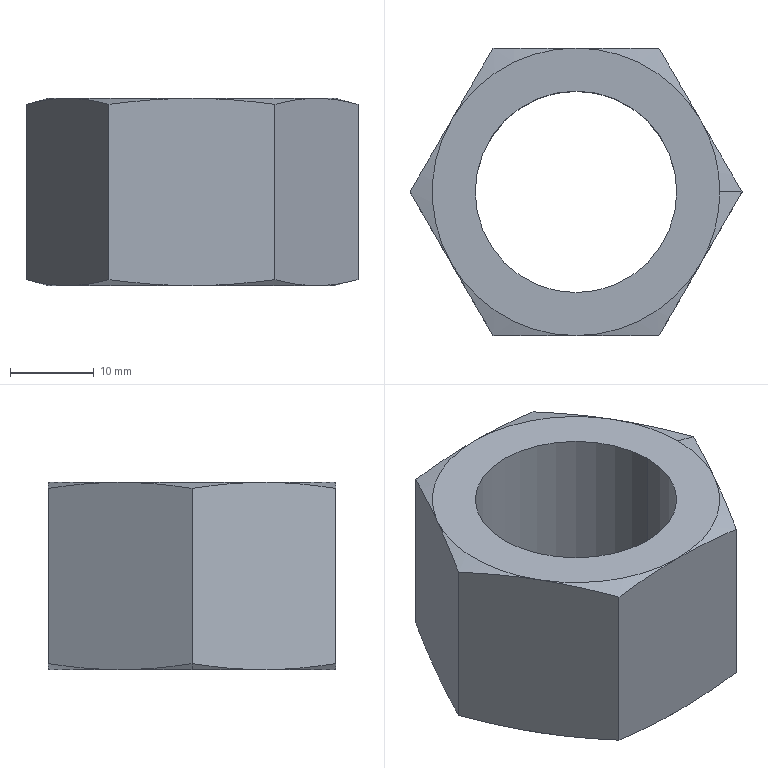Part | SolidWorks | features Cut 2, Chamfer 1, Extrusion 1 | 1 solid | 24 faces | box 39.55 x 34.251 x 22.3 mm | volume 12527 mm3 | cone 14 | plane 8 | cylinder 2 | commonest cylinder face diameters 24 x2
STEP:
#1=CARTESIAN_POINT('',(14.831,8.563,22.3));
#2=VERTEX_POINT('',#1);
#3=CARTESIAN_POINT('',(17.126,0.,22.3));
#4=VERTEX_POINT('',#3);
#5=CARTESIAN_POINT('',(0.,0.,22.3));
#6=DIRECTION('',(0.,0.,-1.));
#7=DIRECTION('',(-1.,0.,0.));
#8=AXIS2_PLACEMENT_3D('',#5,#6,#7);
#9=CIRCLE('',#8,17.126);
#10=EDGE_CURVE('',#2,#4,#9,.T.);
#11=ORIENTED_EDGE('',*,*,#10,.T.);
#12=CARTESIAN_POINT('',(19.775,0.,21.59));
#13=VERTEX_POINT('',#12);
#14=CARTESIAN_POINT('',(17.126,0.,22.3));
#15=DIRECTION('',(0.9659,0.,-0.2588));
#16=VECTOR('',#15,1000.);
#17=LINE('',#14,#16);
#18=EDGE_CURVE('',#4,#13,#17,.T.);
#19=ORIENTED_EDGE('',*,*,#18,.T.);
#20=CARTESIAN_POINT('',(19.775,0.,21.59));
#21=CARTESIAN_POINT('',(18.951,1.427,21.811));
#22=CARTESIAN_POINT('',(18.127,2.854,21.99));
#23=CARTESIAN_POINT('',(16.479,5.709,22.235));
#24=CARTESIAN_POINT('',(15.655,7.136,22.3));
#25=CARTESIAN_POINT('',(14.831,8.563,22.3));
#26=B_SPLINE_CURVE_WITH_KNOTS('',3,(#20,#21,#22,#23,#24,#25),.UNSPECIFIED.,.F.,.F.,(4,2,4),(0.000000231,0.004944,0.009888),.UNSPECIFIED.);
#27=EDGE_CURVE('',#13,#2,#26,.T.);
#28=ORIENTED_EDGE('',*,*,#27,.T.);
#29=EDGE_LOOP('',(#11,#19,#28));
#30=FACE_OUTER_BOUND('',#29,.T.);
#31=CARTESIAN_POINT('',(0.,0.,22.3));
#32=DIRECTION('',(0.,0.,-1.));
#33=DIRECTION('',(1.,0.,0.));
#34=AXIS2_PLACEMENT_3D('',#31,#32,#33);
#35=CONICAL_SURFACE('',#34,17.126,1.309);
#36=ADVANCED_FACE('',(#30),#35,.T.);
#37=CARTESIAN_POINT('',(-17.126,0.,0.));
#38=VERTEX_POINT('',#37);
#39=CARTESIAN_POINT('',(-14.831,8.563,0.));
#40=VERTEX_POINT('',#39);
#41=CARTESIAN_POINT('',(0.,0.,0.));
#42=DIRECTION('',(0.,0.,-1.));
#43=DIRECTION('',(-1.,0.,0.));
#44=AXIS2_PLACEMENT_3D('',#41,#42,#43);
#45=CIRCLE('',#44,17.126);
#46=EDGE_CURVE('',#38,#40,#45,.T.);
#47=ORIENTED_EDGE('',*,*,#46,.F.);
#48=CARTESIAN_POINT('',(-19.775,0.,0.7099));
#49=VERTEX_POINT('',#48);
#50=CARTESIAN_POINT('',(-17.126,0.,0.));
#51=DIRECTION('',(-0.9659,0.,0.2588));
#52=VECTOR('',#51,1000.);
#53=LINE('',#50,#52);
#54=EDGE_CURVE('',#38,#49,#53,.T.);
#55=ORIENTED_EDGE('',*,*,#54,.T.);
#56=CARTESIAN_POINT('',(-19.775,0.,0.7099));
#57=CARTESIAN_POINT('',(-18.951,1.427,0.4891));
#58=CARTESIAN_POINT('',(-18.127,2.854,0.3098));
#59=CARTESIAN_POINT('',(-16.479,5.709,0.06491));
#60=CARTESIAN_POINT('',(-15.655,7.136,0.));
#61=CARTESIAN_POINT('',(-14.831,8.563,0.));
#62=B_SPLINE_CURVE_WITH_KNOTS('',3,(#56,#57,#58,#59,#60,#61),.UNSPECIFIED.,.F.,.F.,(4,2,4),(0.000000231,0.004944,0.009888),.UNSPECIFIED.);
#63=EDGE_CURVE('',#49,#40,#62,.T.);
#64=ORIENTED_EDGE('',*,*,#63,.T.);
#65=EDGE_LOOP('',(#47,#55,#64));
#66=FACE_OUTER_BOUND('',#65,.T.);
#67=CARTESIAN_POINT('',(0.,0.,0.));
#68=DIRECTION('',(0.,0.,1.));
#69=DIRECTION('',(-1.,0.,0.));
#70=AXIS2_PLACEMENT_3D('',#67,#68,#69);
#71=CONICAL_SURFACE('',#70,17.126,1.309);
#72=ADVANCED_FACE('',(#66),#71,.T.);
#73=CARTESIAN_POINT('',(-12.,0.,22.3));
#74=VERTEX_POINT('',#73);
#75=CARTESIAN_POINT('',(12.,0.,22.3));
#76=VERTEX_POINT('',#75);
#77=CARTESIAN_POINT('',(0.,0.,22.3));
#78=DIRECTION('',(0.,0.,1.));
#79=DIRECTION('',(1.,0.,0.));
#80=AXIS2_PLACEMENT_3D('',#77,#78,#79);
#81=CIRCLE('',#80,12.);
#82=EDGE_CURVE('',#74,#76,#81,.T.);
#83=ORIENTED_EDGE('',*,*,#82,.T.);
#84=CARTESIAN_POINT('',(12.,0.,0.));
#85=VERTEX_POINT('',#84);
#86=CARTESIAN_POINT('',(12.,0.,22.3));
#87=DIRECTION('',(0.,0.,-1.));
#88=VECTOR('',#87,1000.);
#89=LINE('',#86,#88);
#90=EDGE_CURVE('',#76,#85,#89,.T.);
#91=ORIENTED_EDGE('',*,*,#90,.T.);
#92=CARTESIAN_POINT('',(-12.,0.,0.));
#93=VERTEX_POINT('',#92);
#94=CARTESIAN_POINT('',(0.,0.,0.));
#95=DIRECTION('',(0.,0.,1.));
#96=DIRECTION('',(1.,0.,0.));
#97=AXIS2_PLACEMENT_3D('',#94,#95,#96);
#98=CIRCLE('',#97,12.);
#99=EDGE_CURVE('',#93,#85,#98,.T.);
#100=ORIENTED_EDGE('',*,*,#99,.F.);
#101=CARTESIAN_POINT('',(-12.,0.,22.3));
#102=DIRECTION('',(0.,0.,-1.));
#103=VECTOR('',#102,1000.);
#104=LINE('',#101,#103);
#105=EDGE_CURVE('',#74,#93,#104,.T.);
#106=ORIENTED_EDGE('',*,*,#105,.F.);
#107=EDGE_LOOP('',(#83,#91,#100,#106));
#108=FACE_OUTER_BOUND('',#107,.T.);
#109=CARTESIAN_POINT('',(0.,0.,22.3));
#110=DIRECTION('',(0.,0.,-1.));
#111=DIRECTION('',(-1.,0.,0.));
#112=AXIS2_PLACEMENT_3D('',#109,#110,#111);
#113=CYLINDRICAL_SURFACE('',#112,12.);
#114=ADVANCED_FACE('',(#108),#113,.F.);
#115=ORIENTED_EDGE('',*,*,#27,.F.);
#116=CARTESIAN_POINT('',(19.775,0.,0.7099));
#117=VERTEX_POINT('',#116);
#118=CARTESIAN_POINT('',(19.775,0.,22.3));
#119=DIRECTION('',(0.,0.,-1.));
#120=VECTOR('',#119,1000.);
#121=LINE('',#118,#120);
#122=EDGE_CURVE('',#13,#117,#121,.T.);
#123=ORIENTED_EDGE('',*,*,#122,.T.);
#124=CARTESIAN_POINT('',(14.831,8.563,0.));
#125=VERTEX_POINT('',#124);
#126=CARTESIAN_POINT('',(14.831,8.563,0.));
#127=CARTESIAN_POINT('',(15.655,7.136,0.));
#128=CARTESIAN_POINT('',(16.479,5.709,0.06491));
#129=CARTESIAN_POINT('',(18.127,2.854,0.3098));
#130=CARTESIAN_POINT('',(18.951,1.427,0.4891));
#131=CARTESIAN_POINT('',(19.775,0.,0.7099));
#132=B_SPLINE_CURVE_WITH_KNOTS('',3,(#126,#127,#128,#129,#130,#131),.UNSPECIFIED.,.F.,.F.,(4,2,4),(0.009888,0.01483,0.01978),.UNSPECIFIED.);
#133=EDGE_CURVE('',#125,#117,#132,.T.);
#134=ORIENTED_EDGE('',*,*,#133,.F.);
#135=CARTESIAN_POINT('',(9.888,17.126,0.7099));
#136=VERTEX_POINT('',#135);
#137=CARTESIAN_POINT('',(9.888,17.126,0.7099));
#138=CARTESIAN_POINT('',(10.711,15.699,0.4891));
#139=CARTESIAN_POINT('',(11.535,14.271,0.3098));
#140=CARTESIAN_POINT('',(13.183,11.417,0.06491));
#141=CARTESIAN_POINT('',(14.007,9.99,0.));
#142=CARTESIAN_POINT('',(14.831,8.563,0.));
#143=B_SPLINE_CURVE_WITH_KNOTS('',3,(#137,#138,#139,#140,#141,#142),.UNSPECIFIED.,.F.,.F.,(4,2,4),(0.000000231,0.004944,0.009888),.UNSPECIFIED.);
#144=EDGE_CURVE('',#136,#125,#143,.T.);
#145=ORIENTED_EDGE('',*,*,#144,.F.);
#146=CARTESIAN_POINT('',(9.888,17.126,21.59));
#147=VERTEX_POINT('',#146);
#148=CARTESIAN_POINT('',(9.888,17.126,22.3));
#149=DIRECTION('',(0.,0.,-1.));
#150=VECTOR('',#149,1000.);
#151=LINE('',#148,#150);
#152=EDGE_CURVE('',#147,#136,#151,.T.);
#153=ORIENTED_EDGE('',*,*,#152,.F.);
#154=CARTESIAN_POINT('',(14.831,8.563,22.3));
#155=CARTESIAN_POINT('',(14.007,9.99,22.3));
#156=CARTESIAN_POINT('',(13.183,11.417,22.235));
#157=CARTESIAN_POINT('',(11.535,14.271,21.99));
#158=CARTESIAN_POINT('',(10.711,15.699,21.811));
#159=CARTESIAN_POINT('',(9.888,17.126,21.59));
#160=B_SPLINE_CURVE_WITH_KNOTS('',3,(#154,#155,#156,#157,#158,#159),.UNSPECIFIED.,.F.,.F.,(4,2,4),(0.009888,0.01483,0.01978),.UNSPECIFIED.);
#161=EDGE_CURVE('',#2,#147,#160,.T.);
#162=ORIENTED_EDGE('',*,*,#161,.F.);
#163=EDGE_LOOP('',(#115,#123,#134,#145,#153,#162));
#164=FACE_OUTER_BOUND('',#163,.T.);
#165=CARTESIAN_POINT('',(19.775,0.,22.3));
#166=DIRECTION('',(-0.866,-0.5,0.));
#167=DIRECTION('',(0.5,-0.866,0.));
#168=AXIS2_PLACEMENT_3D('',#165,#166,#167);
#169=PLANE('',#168);
#170=ADVANCED_FACE('',(#164),#169,.F.);
#171=CARTESIAN_POINT('',(0.,17.126,22.3));
#172=VERTEX_POINT('',#171);
#173=CARTESIAN_POINT('',(9.888,17.126,21.59));
#174=CARTESIAN_POINT('',(8.242,17.126,21.811));
#175=CARTESIAN_POINT('',(6.596,17.126,21.99));
#176=CARTESIAN_POINT('',(3.3,17.126,22.235));
#177=CARTESIAN_POINT('',(1.651,17.126,22.3));
#178=CARTESIAN_POINT('',(0.,17.126,22.3));
#179=B_SPLINE_CURVE_WITH_KNOTS('',3,(#173,#174,#175,#176,#177,#178),.UNSPECIFIED.,.F.,.F.,(4,2,4),(0.05691,0.06188,0.06685),.UNSPECIFIED.);
#180=EDGE_CURVE('',#147,#172,#179,.T.);
#181=ORIENTED_EDGE('',*,*,#180,.F.);
#182=ORIENTED_EDGE('',*,*,#152,.T.);
#183=CARTESIAN_POINT('',(0.,17.126,0.));
#184=VERTEX_POINT('',#183);
#185=CARTESIAN_POINT('',(0.,17.126,0.));
#186=CARTESIAN_POINT('',(1.651,17.126,0.));
#187=CARTESIAN_POINT('',(3.3,17.126,0.06515));
#188=CARTESIAN_POINT('',(6.596,17.126,0.3103));
#189=CARTESIAN_POINT('',(8.242,17.126,0.4895));
#190=CARTESIAN_POINT('',(9.888,17.126,0.7099));
#191=B_SPLINE_CURVE_WITH_KNOTS('',3,(#185,#186,#187,#188,#189,#190),.UNSPECIFIED.,.F.,.F.,(4,2,4),(0.02684,0.03182,0.03681),.UNSPECIFIED.);
#192=EDGE_CURVE('',#184,#136,#191,.T.);
#193=ORIENTED_EDGE('',*,*,#192,.F.);
#194=CARTESIAN_POINT('',(-9.887,17.126,0.7099));
#195=VERTEX_POINT('',#194);
#196=CARTESIAN_POINT('',(-9.887,17.126,0.7099));
#197=CARTESIAN_POINT('',(-8.244,17.126,0.4897));
#198=CARTESIAN_POINT('',(-6.591,17.126,0.3098));
#199=CARTESIAN_POINT('',(-3.293,17.126,0.06475));
#200=CARTESIAN_POINT('',(-1.646,17.126,0.));
#201=CARTESIAN_POINT('',(0.,17.126,0.));
#202=B_SPLINE_CURVE_WITH_KNOTS('',3,(#196,#197,#198,#199,#200,#201),.UNSPECIFIED.,.F.,.F.,(4,2,4),(0.0169,0.02187,0.02684),.UNSPECIFIED.);
#203=EDGE_CURVE('',#195,#184,#202,.T.);
#204=ORIENTED_EDGE('',*,*,#203,.F.);
#205=CARTESIAN_POINT('',(-9.887,17.126,21.59));
#206=VERTEX_POINT('',#205);
#207=CARTESIAN_POINT('',(-9.887,17.126,22.3));
#208=DIRECTION('',(0.,0.,-1.));
#209=VECTOR('',#208,1000.);
#210=LINE('',#207,#209);
#211=EDGE_CURVE('',#206,#195,#210,.T.);
#212=ORIENTED_EDGE('',*,*,#211,.F.);
#213=CARTESIAN_POINT('',(0.,17.126,22.3));
#214=CARTESIAN_POINT('',(-1.646,17.126,22.3));
#215=CARTESIAN_POINT('',(-3.293,17.126,22.235));
#216=CARTESIAN_POINT('',(-6.591,17.126,21.99));
#217=CARTESIAN_POINT('',(-8.244,17.126,21.81));
#218=CARTESIAN_POINT('',(-9.887,17.126,21.59));
#219=B_SPLINE_CURVE_WITH_KNOTS('',3,(#213,#214,#215,#216,#217,#218),.UNSPECIFIED.,.F.,.F.,(4,2,4),(0.06685,0.07181,0.07677),.UNSPECIFIED.);
#220=EDGE_CURVE('',#172,#206,#219,.T.);
#221=ORIENTED_EDGE('',*,*,#220,.F.);
#222=EDGE_LOOP('',(#181,#182,#193,#204,#212,#221));
#223=FACE_OUTER_BOUND('',#222,.T.);
#224=CARTESIAN_POINT('',(9.888,17.126,22.3));
#225=DIRECTION('',(0.,-1.,0.));
#226=DIRECTION('',(1.,0.,0.));
#227=AXIS2_PLACEMENT_3D('',#224,#225,#226);
#228=PLANE('',#227);
#229=ADVANCED_FACE('',(#223),#228,.F.);
#230=CARTESIAN_POINT('',(-14.831,8.563,22.3));
#231=VERTEX_POINT('',#230);
#232=CARTESIAN_POINT('',(-9.887,17.126,21.59));
#233=CARTESIAN_POINT('',(-10.711,15.699,21.811));
#234=CARTESIAN_POINT('',(-11.535,14.271,21.99));
#235=CARTESIAN_POINT('',(-13.183,11.417,22.235));
#236=CARTESIAN_POINT('',(-14.007,9.99,22.3));
#237=CARTESIAN_POINT('',(-14.831,8.563,22.3));
#238=B_SPLINE_CURVE_WITH_KNOTS('',3,(#232,#233,#234,#235,#236,#237),.UNSPECIFIED.,.F.,.F.,(4,2,4),(0.000000231,0.004944,0.009888),.UNSPECIFIED.);
#239=EDGE_CURVE('',#206,#231,#238,.T.);
#240=ORIENTED_EDGE('',*,*,#239,.F.);
#241=ORIENTED_EDGE('',*,*,#211,.T.);
#242=CARTESIAN_POINT('',(-14.831,8.563,0.));
#243=CARTESIAN_POINT('',(-14.007,9.99,0.));
#244=CARTESIAN_POINT('',(-13.183,11.417,0.06491));
#245=CARTESIAN_POINT('',(-11.535,14.271,0.3098));
#246=CARTESIAN_POINT('',(-10.711,15.699,0.4891));
#247=CARTESIAN_POINT('',(-9.887,17.126,0.7099));
#248=B_SPLINE_CURVE_WITH_KNOTS('',3,(#242,#243,#244,#245,#246,#247),.UNSPECIFIED.,.F.,.F.,(4,2,4),(0.009888,0.01483,0.01978),.UNSPECIFIED.);
#249=EDGE_CURVE('',#40,#195,#248,.T.);
#250=ORIENTED_EDGE('',*,*,#249,.F.);
#251=ORIENTED_EDGE('',*,*,#63,.F.);
#252=CARTESIAN_POINT('',(-19.775,0.,21.59));
#253=VERTEX_POINT('',#252);
#254=CARTESIAN_POINT('',(-19.775,0.,22.3));
#255=DIRECTION('',(0.,0.,-1.));
#256=VECTOR('',#255,1000.);
#257=LINE('',#254,#256);
#258=EDGE_CURVE('',#253,#49,#257,.T.);
#259=ORIENTED_EDGE('',*,*,#258,.F.);
#260=CARTESIAN_POINT('',(-14.831,8.563,22.3));
#261=CARTESIAN_POINT('',(-15.655,7.136,22.3));
#262=CARTESIAN_POINT('',(-16.479,5.709,22.235));
#263=CARTESIAN_POINT('',(-18.127,2.854,21.99));
#264=CARTESIAN_POINT('',(-18.951,1.427,21.811));
#265=CARTESIAN_POINT('',(-19.775,0.,21.59));
#266=B_SPLINE_CURVE_WITH_KNOTS('',3,(#260,#261,#262,#263,#264,#265),.UNSPECIFIED.,.F.,.F.,(4,2,4),(0.009888,0.01483,0.01978),.UNSPECIFIED.);
#267=EDGE_CURVE('',#231,#253,#266,.T.);
#268=ORIENTED_EDGE('',*,*,#267,.F.);
#269=EDGE_LOOP('',(#240,#241,#250,#251,#259,#268));
#270=FACE_OUTER_BOUND('',#269,.T.);
#271=CARTESIAN_POINT('',(-9.887,17.126,22.3));
#272=DIRECTION('',(0.866,-0.5,0.));
#273=DIRECTION('',(0.5,0.866,0.));
#274=AXIS2_PLACEMENT_3D('',#271,#272,#273);
#275=PLANE('',#274);
#276=ADVANCED_FACE('',(#270),#275,.F.);
#277=CARTESIAN_POINT('',(-14.831,-8.563,22.3));
#278=VERTEX_POINT('',#277);
#279=CARTESIAN_POINT('',(-19.775,0.,21.59));
#280=CARTESIAN_POINT('',(-18.951,-1.427,21.811));
#281=CARTESIAN_POINT('',(-18.127,-2.854,21.99));
#282=CARTESIAN_POINT('',(-16.479,-5.709,22.235));
#283=CARTESIAN_POINT('',(-15.655,-7.136,22.3));
#284=CARTESIAN_POINT('',(-14.831,-8.563,22.3));
#285=B_SPLINE_CURVE_WITH_KNOTS('',3,(#279,#280,#281,#282,#283,#284),.UNSPECIFIED.,.F.,.F.,(4,2,4),(0.000000231,0.004944,0.009888),.UNSPECIFIED.);
#286=EDGE_CURVE('',#253,#278,#285,.T.);
#287=ORIENTED_EDGE('',*,*,#286,.F.);
#288=ORIENTED_EDGE('',*,*,#258,.T.);
#289=CARTESIAN_POINT('',(-14.831,-8.563,0.));
#290=VERTEX_POINT('',#289);
#291=CARTESIAN_POINT('',(-14.831,-8.563,0.));
#292=CARTESIAN_POINT('',(-15.655,-7.136,0.));
#293=CARTESIAN_POINT('',(-16.479,-5.709,0.06491));
#294=CARTESIAN_POINT('',(-18.127,-2.854,0.3098));
#295=CARTESIAN_POINT('',(-18.951,-1.427,0.4891));
#296=CARTESIAN_POINT('',(-19.775,0.,0.7099));
#297=B_SPLINE_CURVE_WITH_KNOTS('',3,(#291,#292,#293,#294,#295,#296),.UNSPECIFIED.,.F.,.F.,(4,2,4),(0.009888,0.01483,0.01978),.UNSPECIFIED.);
#298=EDGE_CURVE('',#290,#49,#297,.T.);
#299=ORIENTED_EDGE('',*,*,#298,.F.);
#300=CARTESIAN_POINT('',(-9.887,-17.126,0.7099));
#301=VERTEX_POINT('',#300);
#302=CARTESIAN_POINT('',(-9.887,-17.126,0.7099));
#303=CARTESIAN_POINT('',(-10.711,-15.699,0.4891));
#304=CARTESIAN_POINT('',(-11.535,-14.271,0.3098));
#305=CARTESIAN_POINT('',(-13.183,-11.417,0.06491));
#306=CARTESIAN_POINT('',(-14.007,-9.99,0.));
#307=CARTESIAN_POINT('',(-14.831,-8.563,0.));
#308=B_SPLINE_CURVE_WITH_KNOTS('',3,(#302,#303,#304,#305,#306,#307),.UNSPECIFIED.,.F.,.F.,(4,2,4),(0.000000231,0.004944,0.009888),.UNSPECIFIED.);
#309=EDGE_CURVE('',#301,#290,#308,.T.);
#310=ORIENTED_EDGE('',*,*,#309,.F.);
#311=CARTESIAN_POINT('',(-9.887,-17.126,21.59));
#312=VERTEX_POINT('',#311);
#313=CARTESIAN_POINT('',(-9.887,-17.126,22.3));
#314=DIRECTION('',(0.,0.,-1.));
#315=VECTOR('',#314,1000.);
#316=LINE('',#313,#315);
#317=EDGE_CURVE('',#312,#301,#316,.T.);
#318=ORIENTED_EDGE('',*,*,#317,.F.);
#319=CARTESIAN_POINT('',(-14.831,-8.563,22.3));
#320=CARTESIAN_POINT('',(-14.007,-9.99,22.3));
#321=CARTESIAN_POINT('',(-13.183,-11.417,22.235));
#322=CARTESIAN_POINT('',(-11.535,-14.271,21.99));
#323=CARTESIAN_POINT('',(-10.711,-15.699,21.811));
#324=CARTESIAN_POINT('',(-9.887,-17.126,21.59));
#325=B_SPLINE_CURVE_WITH_KNOTS('',3,(#319,#320,#321,#322,#323,#324),.UNSPECIFIED.,.F.,.F.,(4,2,4),(0.009888,0.01483,0.01978),.UNSPECIFIED.);
#326=EDGE_CURVE('',#278,#312,#325,.T.);
#327=ORIENTED_EDGE('',*,*,#326,.F.);
#328=EDGE_LOOP('',(#287,#288,#299,#310,#318,#327));
#329=FACE_OUTER_BOUND('',#328,.T.);
#330=CARTESIAN_POINT('',(-19.775,0.,22.3));
#331=DIRECTION('',(0.866,0.5,0.));
#332=DIRECTION('',(-0.5,0.866,0.));
#333=AXIS2_PLACEMENT_3D('',#330,#331,#332);
#334=PLANE('',#333);
#335=ADVANCED_FACE('',(#329),#334,.F.);
#336=CARTESIAN_POINT('',(0.,-17.126,22.3));
#337=VERTEX_POINT('',#336);
#338=CARTESIAN_POINT('',(-9.887,-17.126,21.59));
#339=CARTESIAN_POINT('',(-8.244,-17.126,21.81));
#340=CARTESIAN_POINT('',(-6.591,-17.126,21.99));
#341=CARTESIAN_POINT('',(-3.293,-17.126,22.235));
#342=CARTESIAN_POINT('',(-1.646,-17.126,22.3));
#343=CARTESIAN_POINT('',(0.,-17.126,22.3));
#344=B_SPLINE_CURVE_WITH_KNOTS('',3,(#338,#339,#340,#341,#342,#343),.UNSPECIFIED.,.F.,.F.,(4,2,4),(0.0169,0.02187,0.02684),.UNSPECIFIED.);
#345=EDGE_CURVE('',#312,#337,#344,.T.);
#346=ORIENTED_EDGE('',*,*,#345,.F.);
#347=ORIENTED_EDGE('',*,*,#317,.T.);
#348=CARTESIAN_POINT('',(0.,-17.126,0.));
#349=VERTEX_POINT('',#348);
#350=CARTESIAN_POINT('',(0.,-17.126,0.));
#351=CARTESIAN_POINT('',(-1.646,-17.126,0.));
#352=CARTESIAN_POINT('',(-3.293,-17.126,0.06475));
#353=CARTESIAN_POINT('',(-6.591,-17.126,0.3098));
#354=CARTESIAN_POINT('',(-8.244,-17.126,0.4897));
#355=CARTESIAN_POINT('',(-9.887,-17.126,0.7099));
#356=B_SPLINE_CURVE_WITH_KNOTS('',3,(#350,#351,#352,#353,#354,#355),.UNSPECIFIED.,.F.,.F.,(4,2,4),(0.06685,0.07181,0.07677),.UNSPECIFIED.);
#357=EDGE_CURVE('',#349,#301,#356,.T.);
#358=ORIENTED_EDGE('',*,*,#357,.F.);
#359=CARTESIAN_POINT('',(9.887,-17.126,0.7099));
#360=VERTEX_POINT('',#359);
#361=CARTESIAN_POINT('',(9.887,-17.126,0.7099));
#362=CARTESIAN_POINT('',(8.242,-17.126,0.4895));
#363=CARTESIAN_POINT('',(6.596,-17.126,0.3103));
#364=CARTESIAN_POINT('',(3.3,-17.126,0.06515));
#365=CARTESIAN_POINT('',(1.651,-17.126,0.));
#366=CARTESIAN_POINT('',(0.,-17.126,0.));
#367=B_SPLINE_CURVE_WITH_KNOTS('',3,(#361,#362,#363,#364,#365,#366),.UNSPECIFIED.,.F.,.F.,(4,2,4),(0.05691,0.06188,0.06685),.UNSPECIFIED.);
#368=EDGE_CURVE('',#360,#349,#367,.T.);
#369=ORIENTED_EDGE('',*,*,#368,.F.);
#370=CARTESIAN_POINT('',(9.887,-17.126,21.59));
#371=VERTEX_POINT('',#370);
#372=CARTESIAN_POINT('',(9.887,-17.126,22.3));
#373=DIRECTION('',(0.,0.,-1.));
#374=VECTOR('',#373,1000.);
#375=LINE('',#372,#374);
#376=EDGE_CURVE('',#371,#360,#375,.T.);
#377=ORIENTED_EDGE('',*,*,#376,.F.);
#378=CARTESIAN_POINT('',(0.,-17.126,22.3));
#379=CARTESIAN_POINT('',(1.651,-17.126,22.3));
#380=CARTESIAN_POINT('',(3.3,-17.126,22.235));
#381=CARTESIAN_POINT('',(6.596,-17.126,21.99));
#382=CARTESIAN_POINT('',(8.242,-17.126,21.811));
#383=CARTESIAN_POINT('',(9.887,-17.126,21.59));
#384=B_SPLINE_CURVE_WITH_KNOTS('',3,(#378,#379,#380,#381,#382,#383),.UNSPECIFIED.,.F.,.F.,(4,2,4),(0.02684,0.03182,0.03681),.UNSPECIFIED.);
#385=EDGE_CURVE('',#337,#371,#384,.T.);
#386=ORIENTED_EDGE('',*,*,#385,.F.);
#387=EDGE_LOOP('',(#346,#347,#358,#369,#377,#386));
#388=FACE_OUTER_BOUND('',#387,.T.);
#389=CARTESIAN_POINT('',(-9.887,-17.126,22.3));
#390=DIRECTION('',(0.,1.,0.));
#391=DIRECTION('',(-1.,0.,0.));
#392=AXIS2_PLACEMENT_3D('',#389,#390,#391);
#393=PLANE('',#392);
#394=ADVANCED_FACE('',(#388),#393,.F.);
#395=CARTESIAN_POINT('',(14.831,-8.563,22.3));
#396=VERTEX_POINT('',#395);
#397=CARTESIAN_POINT('',(9.887,-17.126,21.59));
#398=CARTESIAN_POINT('',(10.711,-15.699,21.811));
#399=CARTESIAN_POINT('',(11.535,-14.271,21.99));
#400=CARTESIAN_POINT('',(13.183,-11.417,22.235));
#401=CARTESIAN_POINT('',(14.007,-9.99,22.3));
#402=CARTESIAN_POINT('',(14.831,-8.563,22.3));
#403=B_SPLINE_CURVE_WITH_KNOTS('',3,(#397,#398,#399,#400,#401,#402),.UNSPECIFIED.,.F.,.F.,(4,2,4),(0.000000231,0.004944,0.009888),.UNSPECIFIED.);
#404=EDGE_CURVE('',#371,#396,#403,.T.);
#405=ORIENTED_EDGE('',*,*,#404,.F.);
#406=ORIENTED_EDGE('',*,*,#376,.T.);
#407=CARTESIAN_POINT('',(14.831,-8.563,0.));
#408=VERTEX_POINT('',#407);
#409=CARTESIAN_POINT('',(14.831,-8.563,0.));
#410=CARTESIAN_POINT('',(14.007,-9.99,0.));
#411=CARTESIAN_POINT('',(13.183,-11.417,0.06491));
#412=CARTESIAN_POINT('',(11.535,-14.271,0.3098));
#413=CARTESIAN_POINT('',(10.711,-15.699,0.4891));
#414=CARTESIAN_POINT('',(9.887,-17.126,0.7099));
#415=B_SPLINE_CURVE_WITH_KNOTS('',3,(#409,#410,#411,#412,#413,#414),.UNSPECIFIED.,.F.,.F.,(4,2,4),(0.009888,0.01483,0.01978),.UNSPECIFIED.);
#416=EDGE_CURVE('',#408,#360,#415,.T.);
#417=ORIENTED_EDGE('',*,*,#416,.F.);
#418=CARTESIAN_POINT('',(19.775,0.,0.7099));
#419=CARTESIAN_POINT('',(18.951,-1.427,0.4891));
#420=CARTESIAN_POINT('',(18.127,-2.854,0.3098));
#421=CARTESIAN_POINT('',(16.479,-5.709,0.06491));
#422=CARTESIAN_POINT('',(15.655,-7.136,0.));
#423=CARTESIAN_POINT('',(14.831,-8.563,0.));
#424=B_SPLINE_CURVE_WITH_KNOTS('',3,(#418,#419,#420,#421,#422,#423),.UNSPECIFIED.,.F.,.F.,(4,2,4),(0.000000231,0.004944,0.009888),.UNSPECIFIED.);
#425=EDGE_CURVE('',#117,#408,#424,.T.);
#426=ORIENTED_EDGE('',*,*,#425,.F.);
#427=ORIENTED_EDGE('',*,*,#122,.F.);
#428=CARTESIAN_POINT('',(14.831,-8.563,22.3));
#429=CARTESIAN_POINT('',(15.655,-7.136,22.3));
#430=CARTESIAN_POINT('',(16.479,-5.709,22.235));
#431=CARTESIAN_POINT('',(18.127,-2.854,21.99));
#432=CARTESIAN_POINT('',(18.951,-1.427,21.811));
#433=CARTESIAN_POINT('',(19.775,0.,21.59));
#434=B_SPLINE_CURVE_WITH_KNOTS('',3,(#428,#429,#430,#431,#432,#433),.UNSPECIFIED.,.F.,.F.,(4,2,4),(0.009888,0.01483,0.01978),.UNSPECIFIED.);
#435=EDGE_CURVE('',#396,#13,#434,.T.);
#436=ORIENTED_EDGE('',*,*,#435,.F.);
#437=EDGE_LOOP('',(#405,#406,#417,#426,#427,#436));
#438=FACE_OUTER_BOUND('',#437,.T.);
#439=CARTESIAN_POINT('',(9.887,-17.126,22.3));
#440=DIRECTION('',(-0.866,0.5,0.));
#441=DIRECTION('',(-0.5,-0.866,0.));
#442=AXIS2_PLACEMENT_3D('',#439,#440,#441);
#443=PLANE('',#442);
#444=ADVANCED_FACE('',(#438),#443,.F.);
#445=ORIENTED_EDGE('',*,*,#82,.F.);
#446=CARTESIAN_POINT('',(0.,0.,22.3));
#447=DIRECTION('',(0.,0.,1.));
#448=DIRECTION('',(1.,0.,0.));
#449=AXIS2_PLACEMENT_3D('',#446,#447,#448);
#450=CIRCLE('',#449,12.);
#451=EDGE_CURVE('',#76,#74,#450,.T.);
#452=ORIENTED_EDGE('',*,*,#451,.F.);
#453=EDGE_LOOP('',(#445,#452));
#454=FACE_BOUND('',#453,.T.);
#455=CARTESIAN_POINT('',(0.,0.,22.3));
#456=DIRECTION('',(0.,0.,-1.));
#457=DIRECTION('',(-1.,0.,0.));
#458=AXIS2_PLACEMENT_3D('',#455,#456,#457);
#459=CIRCLE('',#458,17.126);
#460=EDGE_CURVE('',#231,#172,#459,.T.);
#461=ORIENTED_EDGE('',*,*,#460,.F.);
#462=CARTESIAN_POINT('',(0.,0.,22.3));
#463=DIRECTION('',(0.,0.,-1.));
#464=DIRECTION('',(-1.,0.,0.));
#465=AXIS2_PLACEMENT_3D('',#462,#463,#464);
#466=CIRCLE('',#465,17.126);
#467=EDGE_CURVE('',#278,#231,#466,.T.);
#468=ORIENTED_EDGE('',*,*,#467,.F.);
#469=CARTESIAN_POINT('',(0.,0.,22.3));
#470=DIRECTION('',(0.,0.,-1.));
#471=DIRECTION('',(-1.,0.,0.));
#472=AXIS2_PLACEMENT_3D('',#469,#470,#471);
#473=CIRCLE('',#472,17.126);
#474=EDGE_CURVE('',#337,#278,#473,.T.);
#475=ORIENTED_EDGE('',*,*,#474,.F.);
#476=CARTESIAN_POINT('',(0.,0.,22.3));
#477=DIRECTION('',(0.,0.,-1.));
#478=DIRECTION('',(-1.,0.,0.));
#479=AXIS2_PLACEMENT_3D('',#476,#477,#478);
#480=CIRCLE('',#479,17.126);
#481=EDGE_CURVE('',#396,#337,#480,.T.);
#482=ORIENTED_EDGE('',*,*,#481,.F.);
#483=CARTESIAN_POINT('',(0.,0.,22.3));
#484=DIRECTION('',(0.,0.,-1.));
#485=DIRECTION('',(-1.,0.,0.));
#486=AXIS2_PLACEMENT_3D('',#483,#484,#485);
#487=CIRCLE('',#486,17.126);
#488=EDGE_CURVE('',#4,#396,#487,.T.);
#489=ORIENTED_EDGE('',*,*,#488,.F.);
#490=ORIENTED_EDGE('',*,*,#10,.F.);
#491=CARTESIAN_POINT('',(0.,0.,22.3));
#492=DIRECTION('',(0.,0.,1.));
#493=DIRECTION('',(1.,0.,0.));
#494=AXIS2_PLACEMENT_3D('',#491,#492,#493);
#495=CIRCLE('',#494,17.126);
#496=EDGE_CURVE('',#2,#172,#495,.T.);
#497=ORIENTED_EDGE('',*,*,#496,.T.);
#498=EDGE_LOOP('',(#461,#468,#475,#482,#489,#490,#497));
#499=FACE_OUTER_BOUND('',#498,.T.);
#500=CARTESIAN_POINT('',(19.775,0.,22.3));
#501=DIRECTION('',(0.,0.,-1.));
#502=DIRECTION('',(-1.,0.,0.));
#503=AXIS2_PLACEMENT_3D('',#500,#501,#502);
#504=PLANE('',#503);
#505=ADVANCED_FACE('',(#454,#499),#504,.F.);
#506=ORIENTED_EDGE('',*,*,#99,.T.);
#507=CARTESIAN_POINT('',(0.,0.,0.));
#508=DIRECTION('',(0.,0.,1.));
#509=DIRECTION('',(1.,0.,0.));
#510=AXIS2_PLACEMENT_3D('',#507,#508,#509);
#511=CIRCLE('',#510,12.);
#512=EDGE_CURVE('',#85,#93,#511,.T.);
#513=ORIENTED_EDGE('',*,*,#512,.T.);
#514=EDGE_LOOP('',(#506,#513));
#515=FACE_BOUND('',#514,.T.);
#516=CARTESIAN_POINT('',(0.,0.,0.));
#517=DIRECTION('',(0.,0.,-1.));
#518=DIRECTION('',(-1.,0.,0.));
#519=AXIS2_PLACEMENT_3D('',#516,#517,#518);
#520=CIRCLE('',#519,17.126);
#521=EDGE_CURVE('',#290,#38,#520,.T.);
#522=ORIENTED_EDGE('',*,*,#521,.T.);
#523=ORIENTED_EDGE('',*,*,#46,.T.);
#524=CARTESIAN_POINT('',(0.,0.,0.));
#525=DIRECTION('',(0.,0.,-1.));
#526=DIRECTION('',(-1.,0.,0.));
#527=AXIS2_PLACEMENT_3D('',#524,#525,#526);
#528=CIRCLE('',#527,17.126);
#529=EDGE_CURVE('',#40,#184,#528,.T.);
#530=ORIENTED_EDGE('',*,*,#529,.T.);
#531=CARTESIAN_POINT('',(0.,0.,0.));
#532=DIRECTION('',(0.,0.,-1.));
#533=DIRECTION('',(-1.,0.,0.));
#534=AXIS2_PLACEMENT_3D('',#531,#532,#533);
#535=CIRCLE('',#534,17.126);
#536=EDGE_CURVE('',#184,#125,#535,.T.);
#537=ORIENTED_EDGE('',*,*,#536,.T.);
#538=CARTESIAN_POINT('',(0.,0.,0.));
#539=DIRECTION('',(0.,0.,-1.));
#540=DIRECTION('',(-1.,0.,0.));
#541=AXIS2_PLACEMENT_3D('',#538,#539,#540);
#542=CIRCLE('',#541,17.126);
#543=EDGE_CURVE('',#125,#408,#542,.T.);
#544=ORIENTED_EDGE('',*,*,#543,.T.);
#545=CARTESIAN_POINT('',(0.,0.,0.));
#546=DIRECTION('',(0.,0.,-1.));
#547=DIRECTION('',(-1.,0.,0.));
#548=AXIS2_PLACEMENT_3D('',#545,#546,#547);
#549=CIRCLE('',#548,17.126);
#550=EDGE_CURVE('',#408,#349,#549,.T.);
#551=ORIENTED_EDGE('',*,*,#550,.T.);
#552=CARTESIAN_POINT('',(0.,0.,0.));
#553=DIRECTION('',(0.,0.,-1.));
#554=DIRECTION('',(-1.,0.,0.));
#555=AXIS2_PLACEMENT_3D('',#552,#553,#554);
#556=CIRCLE('',#555,17.126);
#557=EDGE_CURVE('',#349,#290,#556,.T.);
#558=ORIENTED_EDGE('',*,*,#557,.T.);
#559=EDGE_LOOP('',(#522,#523,#530,#537,#544,#551,#558));
#560=FACE_OUTER_BOUND('',#559,.T.);
#561=CARTESIAN_POINT('',(19.775,0.,0.));
#562=DIRECTION('',(0.,0.,-1.));
#563=DIRECTION('',(-1.,0.,0.));
#564=AXIS2_PLACEMENT_3D('',#561,#562,#563);
#565=PLANE('',#564);
#566=ADVANCED_FACE('',(#515,#560),#565,.T.);
#567=ORIENTED_EDGE('',*,*,#90,.F.);
#568=ORIENTED_EDGE('',*,*,#451,.T.);
#569=ORIENTED_EDGE('',*,*,#105,.T.);
#570=ORIENTED_EDGE('',*,*,#512,.F.);
#571=EDGE_LOOP('',(#567,#568,#569,#570));
#572=FACE_OUTER_BOUND('',#571,.T.);
#573=CARTESIAN_POINT('',(0.,0.,22.3));
#574=DIRECTION('',(0.,0.,-1.));
#575=DIRECTION('',(-1.,0.,0.));
#576=AXIS2_PLACEMENT_3D('',#573,#574,#575);
#577=CYLINDRICAL_SURFACE('',#576,12.);
#578=ADVANCED_FACE('',(#572),#577,.F.);
#579=ORIENTED_EDGE('',*,*,#368,.T.);
#580=ORIENTED_EDGE('',*,*,#550,.F.);
#581=ORIENTED_EDGE('',*,*,#416,.T.);
#582=EDGE_LOOP('',(#579,#580,#581));
#583=FACE_OUTER_BOUND('',#582,.T.);
#584=CARTESIAN_POINT('',(0.,0.,0.));
#585=DIRECTION('',(0.,0.,1.));
#586=DIRECTION('',(-1.,0.,0.));
#587=AXIS2_PLACEMENT_3D('',#584,#585,#586);
#588=CONICAL_SURFACE('',#587,17.126,1.309);
#589=ADVANCED_FACE('',(#583),#588,.T.);
#590=ORIENTED_EDGE('',*,*,#133,.T.);
#591=ORIENTED_EDGE('',*,*,#425,.T.);
#592=ORIENTED_EDGE('',*,*,#543,.F.);
#593=EDGE_LOOP('',(#590,#591,#592));
#594=FACE_OUTER_BOUND('',#593,.T.);
#595=CARTESIAN_POINT('',(0.,0.,0.));
#596=DIRECTION('',(0.,0.,1.));
#597=DIRECTION('',(-1.,0.,0.));
#598=AXIS2_PLACEMENT_3D('',#595,#596,#597);
#599=CONICAL_SURFACE('',#598,17.126,1.309);
#600=ADVANCED_FACE('',(#594),#599,.T.);
#601=ORIENTED_EDGE('',*,*,#309,.T.);
#602=ORIENTED_EDGE('',*,*,#557,.F.);
#603=ORIENTED_EDGE('',*,*,#357,.T.);
#604=EDGE_LOOP('',(#601,#602,#603));
#605=FACE_OUTER_BOUND('',#604,.T.);
#606=CARTESIAN_POINT('',(0.,0.,0.));
#607=DIRECTION('',(0.,0.,1.));
#608=DIRECTION('',(-1.,0.,0.));
#609=AXIS2_PLACEMENT_3D('',#606,#607,#608);
#610=CONICAL_SURFACE('',#609,17.126,1.309);
#611=ADVANCED_FACE('',(#605),#610,.T.);
#612=ORIENTED_EDGE('',*,*,#54,.F.);
#613=ORIENTED_EDGE('',*,*,#521,.F.);
#614=ORIENTED_EDGE('',*,*,#298,.T.);
#615=EDGE_LOOP('',(#612,#613,#614));
#616=FACE_OUTER_BOUND('',#615,.T.);
#617=CARTESIAN_POINT('',(0.,0.,0.));
#618=DIRECTION('',(0.,0.,1.));
#619=DIRECTION('',(-1.,0.,0.));
#620=AXIS2_PLACEMENT_3D('',#617,#618,#619);
#621=CONICAL_SURFACE('',#620,17.126,1.309);
#622=ADVANCED_FACE('',(#616),#621,.T.);
#623=ORIENTED_EDGE('',*,*,#249,.T.);
#624=ORIENTED_EDGE('',*,*,#203,.T.);
#625=ORIENTED_EDGE('',*,*,#529,.F.);
#626=EDGE_LOOP('',(#623,#624,#625));
#627=FACE_OUTER_BOUND('',#626,.T.);
#628=CARTESIAN_POINT('',(0.,0.,0.));
#629=DIRECTION('',(0.,0.,1.));
#630=DIRECTION('',(-1.,0.,0.));
#631=AXIS2_PLACEMENT_3D('',#628,#629,#630);
#632=CONICAL_SURFACE('',#631,17.126,1.309);
#633=ADVANCED_FACE('',(#627),#632,.T.);
#634=ORIENTED_EDGE('',*,*,#192,.T.);
#635=ORIENTED_EDGE('',*,*,#144,.T.);
#636=ORIENTED_EDGE('',*,*,#536,.F.);
#637=EDGE_LOOP('',(#634,#635,#636));
#638=FACE_OUTER_BOUND('',#637,.T.);
#639=CARTESIAN_POINT('',(0.,0.,0.));
#640=DIRECTION('',(0.,0.,1.));
#641=DIRECTION('',(-1.,0.,0.));
#642=AXIS2_PLACEMENT_3D('',#639,#640,#641);
#643=CONICAL_SURFACE('',#642,17.126,1.309);
#644=ADVANCED_FACE('',(#638),#643,.T.);
#645=ORIENTED_EDGE('',*,*,#267,.T.);
#646=ORIENTED_EDGE('',*,*,#286,.T.);
#647=ORIENTED_EDGE('',*,*,#467,.T.);
#648=EDGE_LOOP('',(#645,#646,#647));
#649=FACE_OUTER_BOUND('',#648,.T.);
#650=CARTESIAN_POINT('',(0.,0.,22.3));
#651=DIRECTION('',(0.,0.,-1.));
#652=DIRECTION('',(1.,0.,0.));
#653=AXIS2_PLACEMENT_3D('',#650,#651,#652);
#654=CONICAL_SURFACE('',#653,17.126,1.309);
#655=ADVANCED_FACE('',(#649),#654,.T.);
#656=ORIENTED_EDGE('',*,*,#326,.T.);
#657=ORIENTED_EDGE('',*,*,#345,.T.);
#658=ORIENTED_EDGE('',*,*,#474,.T.);
#659=EDGE_LOOP('',(#656,#657,#658));
#660=FACE_OUTER_BOUND('',#659,.T.);
#661=CARTESIAN_POINT('',(0.,0.,22.3));
#662=DIRECTION('',(0.,0.,-1.));
#663=DIRECTION('',(1.,0.,0.));
#664=AXIS2_PLACEMENT_3D('',#661,#662,#663);
#665=CONICAL_SURFACE('',#664,17.126,1.309);
#666=ADVANCED_FACE('',(#660),#665,.T.);
#667=ORIENTED_EDGE('',*,*,#385,.T.);
#668=ORIENTED_EDGE('',*,*,#404,.T.);
#669=ORIENTED_EDGE('',*,*,#481,.T.);
#670=EDGE_LOOP('',(#667,#668,#669));
#671=FACE_OUTER_BOUND('',#670,.T.);
#672=CARTESIAN_POINT('',(0.,0.,22.3));
#673=DIRECTION('',(0.,0.,-1.));
#674=DIRECTION('',(1.,0.,0.));
#675=AXIS2_PLACEMENT_3D('',#672,#673,#674);
#676=CONICAL_SURFACE('',#675,17.126,1.309);
#677=ADVANCED_FACE('',(#671),#676,.T.);
#678=ORIENTED_EDGE('',*,*,#18,.F.);
#679=ORIENTED_EDGE('',*,*,#488,.T.);
#680=ORIENTED_EDGE('',*,*,#435,.T.);
#681=EDGE_LOOP('',(#678,#679,#680));
#682=FACE_OUTER_BOUND('',#681,.T.);
#683=CARTESIAN_POINT('',(0.,0.,22.3));
#684=DIRECTION('',(0.,0.,-1.));
#685=DIRECTION('',(1.,0.,0.));
#686=AXIS2_PLACEMENT_3D('',#683,#684,#685);
#687=CONICAL_SURFACE('',#686,17.126,1.309);
#688=ADVANCED_FACE('',(#682),#687,.T.);
#689=ORIENTED_EDGE('',*,*,#161,.T.);
#690=ORIENTED_EDGE('',*,*,#180,.T.);
#691=ORIENTED_EDGE('',*,*,#496,.F.);
#692=EDGE_LOOP('',(#689,#690,#691));
#693=FACE_OUTER_BOUND('',#692,.T.);
#694=CARTESIAN_POINT('',(0.,0.,22.3));
#695=DIRECTION('',(0.,0.,-1.));
#696=DIRECTION('',(1.,0.,0.));
#697=AXIS2_PLACEMENT_3D('',#694,#695,#696);
#698=CONICAL_SURFACE('',#697,17.126,1.309);
#699=ADVANCED_FACE('',(#693),#698,.T.);
#700=ORIENTED_EDGE('',*,*,#220,.T.);
#701=ORIENTED_EDGE('',*,*,#239,.T.);
#702=ORIENTED_EDGE('',*,*,#460,.T.);
#703=EDGE_LOOP('',(#700,#701,#702));
#704=FACE_OUTER_BOUND('',#703,.T.);
#705=CARTESIAN_POINT('',(0.,0.,22.3));
#706=DIRECTION('',(0.,0.,-1.));
#707=DIRECTION('',(1.,0.,0.));
#708=AXIS2_PLACEMENT_3D('',#705,#706,#707);
#709=CONICAL_SURFACE('',#708,17.126,1.309);
#710=ADVANCED_FACE('',(#704),#709,.T.);
#711=CLOSED_SHELL('',(#36,#72,#114,#170,#229,#276,#335,#394,#444,#505,#566,#578,#589,#600,#611,#622,#633,#644,#655,#666,#677,#688,#699,#710));
#712=MANIFOLD_SOLID_BREP('',#711);
#713=CARTESIAN_POINT('',(0.,0.,0.));
#714=DIRECTION('',(0.,0.,1.));
#715=DIRECTION('',(1.,0.,0.));
#716=AXIS2_PLACEMENT_3D('',#713,#714,#715);
#717=(LENGTH_UNIT()NAMED_UNIT(*)SI_UNIT(.MILLI.,.METRE.));
#718=UNCERTAINTY_MEASURE_WITH_UNIT(LENGTH_MEASURE(0.00001),#717,'','');
#719=(NAMED_UNIT(*)PLANE_ANGLE_UNIT()SI_UNIT($,.RADIAN.));
#720=(NAMED_UNIT(*)SI_UNIT($,.STERADIAN.)SOLID_ANGLE_UNIT());
#721=(GEOMETRIC_REPRESENTATION_CONTEXT(3)GLOBAL_UNCERTAINTY_ASSIGNED_CONTEXT((#718))GLOBAL_UNIT_ASSIGNED_CONTEXT((#717,#719,#720))REPRESENTATION_CONTEXT('',''));
#722=ADVANCED_BREP_SHAPE_REPRESENTATION('',(#712,#716),#721);